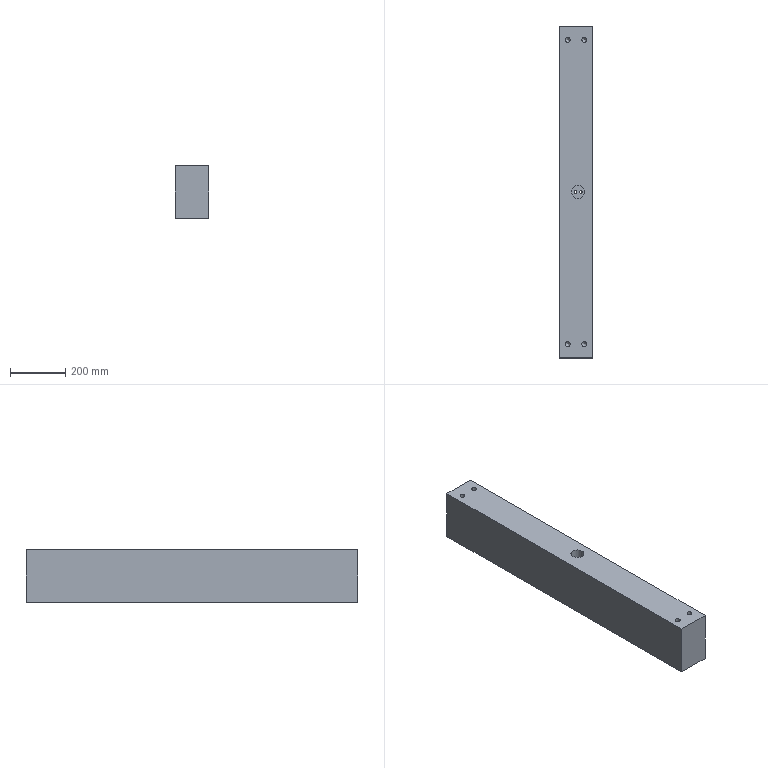Part | STEP file | lll_id4618_x_t | 1 solid | 30 faces | box 120 x 1200 x 190 mm | volume 27062039 mm3 | cylinder 13 | plane 9 | cone 8 | commonest cylinder face diameters 17.506 x8 9 x2 14 x2 47 x1
STEP:
#1=CARTESIAN_POINT('',(2746.188,550.,-370.));
#2=VERTEX_POINT('',#1);
#3=CARTESIAN_POINT('',(2737.435,550.,-370.));
#4=DIRECTION('',(0.,0.,1.));
#5=DIRECTION('',(1.,0.,0.));
#6=AXIS2_PLACEMENT_3D('',#3,#4,#5);
#7=CIRCLE('',#6,8.753);
#8=EDGE_CURVE('',#2,#2,#7,.T.);
#9=ORIENTED_EDGE('',*,*,#8,.T.);
#10=EDGE_LOOP('',(#9));
#11=FACE_BOUND('',#10,.T.);
#12=CARTESIAN_POINT('',(2746.188,-550.,-370.));
#13=VERTEX_POINT('',#12);
#14=CARTESIAN_POINT('',(2737.435,-550.,-370.));
#15=DIRECTION('',(0.,0.,1.));
#16=DIRECTION('',(1.,0.,0.));
#17=AXIS2_PLACEMENT_3D('',#14,#15,#16);
#18=CIRCLE('',#17,8.753);
#19=EDGE_CURVE('',#13,#13,#18,.T.);
#20=ORIENTED_EDGE('',*,*,#19,.T.);
#21=EDGE_LOOP('',(#20));
#22=FACE_BOUND('',#21,.T.);
#23=CARTESIAN_POINT('',(2698.,0.,-370.));
#24=VERTEX_POINT('',#23);
#25=CARTESIAN_POINT('',(2705.,0.,-370.));
#26=DIRECTION('',(0.,0.,1.));
#27=DIRECTION('',(-1.,0.,0.));
#28=AXIS2_PLACEMENT_3D('',#25,#26,#27);
#29=CIRCLE('',#28,7.);
#30=EDGE_CURVE('',#24,#24,#29,.T.);
#31=ORIENTED_EDGE('',*,*,#30,.T.);
#32=EDGE_LOOP('',(#31));
#33=FACE_BOUND('',#32,.T.);
#34=CARTESIAN_POINT('',(2647.435,600.,-370.));
#35=VERTEX_POINT('',#34);
#36=CARTESIAN_POINT('',(2647.435,-600.,-370.));
#37=VERTEX_POINT('',#36);
#38=CARTESIAN_POINT('',(2647.435,1.,-370.));
#39=DIRECTION('',(0.,-1.,0.));
#40=VECTOR('',#39,1.);
#41=LINE('',#38,#40);
#42=EDGE_CURVE('',#35,#37,#41,.T.);
#43=ORIENTED_EDGE('',*,*,#42,.F.);
#44=CARTESIAN_POINT('',(2767.435,600.,-370.));
#45=VERTEX_POINT('',#44);
#46=CARTESIAN_POINT('',(-1202.565,600.,-370.));
#47=DIRECTION('',(1.,0.,0.));
#48=VECTOR('',#47,1.);
#49=LINE('',#46,#48);
#50=EDGE_CURVE('',#35,#45,#49,.T.);
#51=ORIENTED_EDGE('',*,*,#50,.T.);
#52=CARTESIAN_POINT('',(2767.435,-600.,-370.));
#53=VERTEX_POINT('',#52);
#54=CARTESIAN_POINT('',(2767.435,600.,-370.));
#55=DIRECTION('',(0.,-1.,0.));
#56=VECTOR('',#55,1.);
#57=LINE('',#54,#56);
#58=EDGE_CURVE('',#45,#53,#57,.T.);
#59=ORIENTED_EDGE('',*,*,#58,.T.);
#60=CARTESIAN_POINT('',(2767.435,-600.,-370.));
#61=DIRECTION('',(-1.,0.,0.));
#62=VECTOR('',#61,1.);
#63=LINE('',#60,#62);
#64=EDGE_CURVE('',#53,#37,#63,.T.);
#65=ORIENTED_EDGE('',*,*,#64,.T.);
#66=EDGE_LOOP('',(#43,#51,#59,#65));
#67=FACE_BOUND('',#66,.T.);
#68=CARTESIAN_POINT('',(2718.,0.,-370.));
#69=VERTEX_POINT('',#68);
#70=CARTESIAN_POINT('',(2725.,0.,-370.));
#71=DIRECTION('',(0.,0.,1.));
#72=DIRECTION('',(-1.,0.,0.));
#73=AXIS2_PLACEMENT_3D('',#70,#71,#72);
#74=CIRCLE('',#73,7.);
#75=EDGE_CURVE('',#69,#69,#74,.T.);
#76=ORIENTED_EDGE('',*,*,#75,.T.);
#77=EDGE_LOOP('',(#76));
#78=FACE_BOUND('',#77,.T.);
#79=CARTESIAN_POINT('',(2686.188,550.,-370.));
#80=VERTEX_POINT('',#79);
#81=CARTESIAN_POINT('',(2677.435,550.,-370.));
#82=DIRECTION('',(0.,0.,1.));
#83=DIRECTION('',(1.,0.,0.));
#84=AXIS2_PLACEMENT_3D('',#81,#82,#83);
#85=CIRCLE('',#84,8.753);
#86=EDGE_CURVE('',#80,#80,#85,.T.);
#87=ORIENTED_EDGE('',*,*,#86,.T.);
#88=EDGE_LOOP('',(#87));
#89=FACE_BOUND('',#88,.T.);
#90=CARTESIAN_POINT('',(2686.188,-550.,-370.));
#91=VERTEX_POINT('',#90);
#92=CARTESIAN_POINT('',(2677.435,-550.,-370.));
#93=DIRECTION('',(0.,0.,1.));
#94=DIRECTION('',(1.,0.,0.));
#95=AXIS2_PLACEMENT_3D('',#92,#93,#94);
#96=CIRCLE('',#95,8.753);
#97=EDGE_CURVE('',#91,#91,#96,.T.);
#98=ORIENTED_EDGE('',*,*,#97,.T.);
#99=EDGE_LOOP('',(#98));
#100=FACE_BOUND('',#99,.T.);
#101=CARTESIAN_POINT('',(4953.751,1.,-370.));
#102=DIRECTION('',(0.,0.,-1.));
#103=DIRECTION('',(-1.,0.,0.));
#104=AXIS2_PLACEMENT_3D('',#101,#102,#103);
#105=PLANE('',#104);
#106=ADVANCED_FACE('',(#11,#22,#33,#67,#78,#89,#100),#105,.T.);
#107=CARTESIAN_POINT('',(2720.5,0.,-292.));
#108=VERTEX_POINT('',#107);
#109=CARTESIAN_POINT('',(2725.,0.,-292.));
#110=DIRECTION('',(0.,0.,-1.));
#111=DIRECTION('',(-1.,0.,0.));
#112=AXIS2_PLACEMENT_3D('',#109,#110,#111);
#113=CIRCLE('',#112,4.5);
#114=EDGE_CURVE('',#108,#108,#113,.T.);
#115=ORIENTED_EDGE('',*,*,#114,.F.);
#116=EDGE_LOOP('',(#115));
#117=FACE_BOUND('',#116,.T.);
#118=CARTESIAN_POINT('',(2720.5,0.,-322.));
#119=VERTEX_POINT('',#118);
#120=CARTESIAN_POINT('',(2725.,0.,-322.));
#121=DIRECTION('',(0.,0.,-1.));
#122=DIRECTION('',(-1.,0.,0.));
#123=AXIS2_PLACEMENT_3D('',#120,#121,#122);
#124=CIRCLE('',#123,4.5);
#125=EDGE_CURVE('',#119,#119,#124,.T.);
#126=ORIENTED_EDGE('',*,*,#125,.T.);
#127=EDGE_LOOP('',(#126));
#128=FACE_BOUND('',#127,.T.);
#129=CARTESIAN_POINT('',(2725.,0.,-432.));
#130=DIRECTION('',(0.,0.,1.));
#131=DIRECTION('',(1.,0.,0.));
#132=AXIS2_PLACEMENT_3D('',#129,#130,#131);
#133=CYLINDRICAL_SURFACE('',#132,4.5);
#134=ADVANCED_FACE('',(#117,#128),#133,.F.);
#135=CARTESIAN_POINT('',(2700.5,0.,-292.));
#136=VERTEX_POINT('',#135);
#137=CARTESIAN_POINT('',(2705.,0.,-292.));
#138=DIRECTION('',(0.,0.,1.));
#139=DIRECTION('',(-1.,0.,0.));
#140=AXIS2_PLACEMENT_3D('',#137,#138,#139);
#141=CIRCLE('',#140,4.5);
#142=EDGE_CURVE('',#136,#136,#141,.T.);
#143=ORIENTED_EDGE('',*,*,#142,.T.);
#144=EDGE_LOOP('',(#143));
#145=FACE_BOUND('',#144,.T.);
#146=CARTESIAN_POINT('',(2700.5,0.,-322.));
#147=VERTEX_POINT('',#146);
#148=CARTESIAN_POINT('',(2705.,0.,-322.));
#149=DIRECTION('',(0.,0.,1.));
#150=DIRECTION('',(-1.,0.,0.));
#151=AXIS2_PLACEMENT_3D('',#148,#149,#150);
#152=CIRCLE('',#151,4.5);
#153=EDGE_CURVE('',#147,#147,#152,.T.);
#154=ORIENTED_EDGE('',*,*,#153,.F.);
#155=EDGE_LOOP('',(#154));
#156=FACE_BOUND('',#155,.T.);
#157=CARTESIAN_POINT('',(2705.,0.,-432.));
#158=DIRECTION('',(0.,0.,1.));
#159=DIRECTION('',(1.,0.,0.));
#160=AXIS2_PLACEMENT_3D('',#157,#158,#159);
#161=CYLINDRICAL_SURFACE('',#160,4.5);
#162=ADVANCED_FACE('',(#145,#156),#161,.F.);
#163=CARTESIAN_POINT('',(2691.5,0.,-292.));
#164=VERTEX_POINT('',#163);
#165=CARTESIAN_POINT('',(2715.,0.,-292.));
#166=DIRECTION('',(0.,0.,-1.));
#167=DIRECTION('',(-1.,0.,0.));
#168=AXIS2_PLACEMENT_3D('',#165,#166,#167);
#169=CIRCLE('',#168,23.5);
#170=EDGE_CURVE('',#164,#164,#169,.T.);
#171=ORIENTED_EDGE('',*,*,#170,.F.);
#172=EDGE_LOOP('',(#171));
#173=FACE_BOUND('',#172,.T.);
#174=ORIENTED_EDGE('',*,*,#142,.F.);
#175=EDGE_LOOP('',(#174));
#176=FACE_BOUND('',#175,.T.);
#177=ORIENTED_EDGE('',*,*,#114,.T.);
#178=EDGE_LOOP('',(#177));
#179=FACE_BOUND('',#178,.T.);
#180=CARTESIAN_POINT('',(2725.8,0.,-292.));
#181=DIRECTION('',(0.,0.,-1.));
#182=DIRECTION('',(1.,0.,0.));
#183=AXIS2_PLACEMENT_3D('',#180,#181,#182);
#184=PLANE('',#183);
#185=ADVANCED_FACE('',(#173,#176,#179),#184,.F.);
#186=CARTESIAN_POINT('',(2668.682,550.,-180.));
#187=VERTEX_POINT('',#186);
#188=CARTESIAN_POINT('',(2677.435,550.,-180.));
#189=DIRECTION('',(0.,0.,-1.));
#190=DIRECTION('',(-1.,0.,0.));
#191=AXIS2_PLACEMENT_3D('',#188,#189,#190);
#192=CIRCLE('',#191,8.753);
#193=EDGE_CURVE('',#187,#187,#192,.T.);
#194=ORIENTED_EDGE('',*,*,#193,.T.);
#195=EDGE_LOOP('',(#194));
#196=FACE_BOUND('',#195,.T.);
#197=CARTESIAN_POINT('',(2668.682,-550.,-180.));
#198=VERTEX_POINT('',#197);
#199=CARTESIAN_POINT('',(2677.435,-550.,-180.));
#200=DIRECTION('',(0.,0.,-1.));
#201=DIRECTION('',(-1.,0.,0.));
#202=AXIS2_PLACEMENT_3D('',#199,#200,#201);
#203=CIRCLE('',#202,8.753);
#204=EDGE_CURVE('',#198,#198,#203,.T.);
#205=ORIENTED_EDGE('',*,*,#204,.T.);
#206=EDGE_LOOP('',(#205));
#207=FACE_BOUND('',#206,.T.);
#208=CARTESIAN_POINT('',(2728.682,-550.,-180.));
#209=VERTEX_POINT('',#208);
#210=CARTESIAN_POINT('',(2737.435,-550.,-180.));
#211=DIRECTION('',(0.,0.,-1.));
#212=DIRECTION('',(-1.,0.,0.));
#213=AXIS2_PLACEMENT_3D('',#210,#211,#212);
#214=CIRCLE('',#213,8.753);
#215=EDGE_CURVE('',#209,#209,#214,.T.);
#216=ORIENTED_EDGE('',*,*,#215,.T.);
#217=EDGE_LOOP('',(#216));
#218=FACE_BOUND('',#217,.T.);
#219=CARTESIAN_POINT('',(2728.682,550.,-180.));
#220=VERTEX_POINT('',#219);
#221=CARTESIAN_POINT('',(2737.435,550.,-180.));
#222=DIRECTION('',(0.,0.,-1.));
#223=DIRECTION('',(-1.,0.,0.));
#224=AXIS2_PLACEMENT_3D('',#221,#222,#223);
#225=CIRCLE('',#224,8.753);
#226=EDGE_CURVE('',#220,#220,#225,.T.);
#227=ORIENTED_EDGE('',*,*,#226,.T.);
#228=EDGE_LOOP('',(#227));
#229=FACE_BOUND('',#228,.T.);
#230=CARTESIAN_POINT('',(2647.435,600.,-180.));
#231=VERTEX_POINT('',#230);
#232=CARTESIAN_POINT('',(2767.435,600.,-180.));
#233=VERTEX_POINT('',#232);
#234=CARTESIAN_POINT('',(4953.751,600.,-180.));
#235=DIRECTION('',(1.,0.,0.));
#236=VECTOR('',#235,1.);
#237=LINE('',#234,#236);
#238=EDGE_CURVE('',#231,#233,#237,.T.);
#239=ORIENTED_EDGE('',*,*,#238,.F.);
#240=CARTESIAN_POINT('',(2647.435,-600.,-180.));
#241=VERTEX_POINT('',#240);
#242=CARTESIAN_POINT('',(2647.435,0.,-180.));
#243=DIRECTION('',(0.,1.,0.));
#244=VECTOR('',#243,1.);
#245=LINE('',#242,#244);
#246=EDGE_CURVE('',#241,#231,#245,.T.);
#247=ORIENTED_EDGE('',*,*,#246,.F.);
#248=CARTESIAN_POINT('',(2767.435,-600.,-180.));
#249=VERTEX_POINT('',#248);
#250=CARTESIAN_POINT('',(4953.751,-600.,-180.));
#251=DIRECTION('',(-1.,0.,0.));
#252=VECTOR('',#251,1.);
#253=LINE('',#250,#252);
#254=EDGE_CURVE('',#249,#241,#253,.T.);
#255=ORIENTED_EDGE('',*,*,#254,.F.);
#256=CARTESIAN_POINT('',(2767.435,1.,-180.));
#257=DIRECTION('',(0.,-1.,0.));
#258=VECTOR('',#257,1.);
#259=LINE('',#256,#258);
#260=EDGE_CURVE('',#233,#249,#259,.T.);
#261=ORIENTED_EDGE('',*,*,#260,.F.);
#262=EDGE_LOOP('',(#239,#247,#255,#261));
#263=FACE_BOUND('',#262,.T.);
#264=CARTESIAN_POINT('',(2691.5,0.,-180.));
#265=VERTEX_POINT('',#264);
#266=CARTESIAN_POINT('',(2715.,0.,-180.));
#267=DIRECTION('',(0.,0.,1.));
#268=DIRECTION('',(-1.,0.,0.));
#269=AXIS2_PLACEMENT_3D('',#266,#267,#268);
#270=CIRCLE('',#269,23.5);
#271=EDGE_CURVE('',#265,#265,#270,.T.);
#272=ORIENTED_EDGE('',*,*,#271,.F.);
#273=EDGE_LOOP('',(#272));
#274=FACE_BOUND('',#273,.T.);
#275=CARTESIAN_POINT('',(4953.751,1.,-180.));
#276=DIRECTION('',(0.,0.,-1.));
#277=DIRECTION('',(-1.,0.,0.));
#278=AXIS2_PLACEMENT_3D('',#275,#276,#277);
#279=PLANE('',#278);
#280=ADVANCED_FACE('',(#196,#207,#218,#229,#263,#274),#279,.F.);
#281=ORIENTED_EDGE('',*,*,#58,.F.);
#282=CARTESIAN_POINT('',(2767.435,600.,-182.5));
#283=DIRECTION('',(0.,0.,-1.));
#284=VECTOR('',#283,1.);
#285=LINE('',#282,#284);
#286=EDGE_CURVE('',#233,#45,#285,.T.);
#287=ORIENTED_EDGE('',*,*,#286,.F.);
#288=ORIENTED_EDGE('',*,*,#260,.T.);
#289=CARTESIAN_POINT('',(2767.435,-600.,-182.5));
#290=DIRECTION('',(0.,0.,-1.));
#291=VECTOR('',#290,1.);
#292=LINE('',#289,#291);
#293=EDGE_CURVE('',#249,#53,#292,.T.);
#294=ORIENTED_EDGE('',*,*,#293,.T.);
#295=EDGE_LOOP('',(#281,#287,#288,#294));
#296=FACE_OUTER_BOUND('',#295,.T.);
#297=CARTESIAN_POINT('',(2767.435,600.,-182.5));
#298=DIRECTION('',(1.,0.,0.));
#299=DIRECTION('',(0.,0.,-1.));
#300=AXIS2_PLACEMENT_3D('',#297,#298,#299);
#301=PLANE('',#300);
#302=ADVANCED_FACE('',(#296),#301,.T.);
#303=CARTESIAN_POINT('',(2647.435,-600.,-251.25));
#304=DIRECTION('',(0.,0.,-1.));
#305=VECTOR('',#304,1.);
#306=LINE('',#303,#305);
#307=EDGE_CURVE('',#241,#37,#306,.T.);
#308=ORIENTED_EDGE('',*,*,#307,.T.);
#309=ORIENTED_EDGE('',*,*,#64,.F.);
#310=ORIENTED_EDGE('',*,*,#293,.F.);
#311=ORIENTED_EDGE('',*,*,#254,.T.);
#312=EDGE_LOOP('',(#308,#309,#310,#311));
#313=FACE_OUTER_BOUND('',#312,.T.);
#314=CARTESIAN_POINT('',(2767.435,-600.,-182.5));
#315=DIRECTION('',(0.,-1.,0.));
#316=DIRECTION('',(0.,0.,-1.));
#317=AXIS2_PLACEMENT_3D('',#314,#315,#316);
#318=PLANE('',#317);
#319=ADVANCED_FACE('',(#313),#318,.T.);
#320=CARTESIAN_POINT('',(2647.435,600.,-251.25));
#321=DIRECTION('',(0.,0.,1.));
#322=VECTOR('',#321,1.);
#323=LINE('',#320,#322);
#324=EDGE_CURVE('',#35,#231,#323,.T.);
#325=ORIENTED_EDGE('',*,*,#324,.T.);
#326=ORIENTED_EDGE('',*,*,#238,.T.);
#327=ORIENTED_EDGE('',*,*,#286,.T.);
#328=ORIENTED_EDGE('',*,*,#50,.F.);
#329=EDGE_LOOP('',(#325,#326,#327,#328));
#330=FACE_OUTER_BOUND('',#329,.T.);
#331=CARTESIAN_POINT('',(-1202.565,600.,-182.5));
#332=DIRECTION('',(0.,1.,0.));
#333=DIRECTION('',(0.,0.,1.));
#334=AXIS2_PLACEMENT_3D('',#331,#332,#333);
#335=PLANE('',#334);
#336=ADVANCED_FACE('',(#330),#335,.T.);
#337=ORIENTED_EDGE('',*,*,#324,.F.);
#338=ORIENTED_EDGE('',*,*,#42,.T.);
#339=ORIENTED_EDGE('',*,*,#307,.F.);
#340=ORIENTED_EDGE('',*,*,#246,.T.);
#341=EDGE_LOOP('',(#337,#338,#339,#340));
#342=FACE_OUTER_BOUND('',#341,.T.);
#343=CARTESIAN_POINT('',(2647.435,0.,-251.25));
#344=DIRECTION('',(1.,0.,0.));
#345=DIRECTION('',(0.,0.,-1.));
#346=AXIS2_PLACEMENT_3D('',#343,#344,#345);
#347=PLANE('',#346);
#348=ADVANCED_FACE('',(#342),#347,.F.);
#349=ORIENTED_EDGE('',*,*,#170,.T.);
#350=EDGE_LOOP('',(#349));
#351=FACE_BOUND('',#350,.T.);
#352=ORIENTED_EDGE('',*,*,#271,.T.);
#353=EDGE_LOOP('',(#352));
#354=FACE_BOUND('',#353,.T.);
#355=CARTESIAN_POINT('',(2715.,0.,-288.));
#356=DIRECTION('',(0.,0.,1.));
#357=DIRECTION('',(1.,0.,0.));
#358=AXIS2_PLACEMENT_3D('',#355,#356,#357);
#359=CYLINDRICAL_SURFACE('',#358,23.5);
#360=ADVANCED_FACE('',(#351,#354),#359,.F.);
#361=CARTESIAN_POINT('',(2698.,0.,-322.));
#362=VERTEX_POINT('',#361);
#363=CARTESIAN_POINT('',(2705.,0.,-322.));
#364=DIRECTION('',(0.,0.,1.));
#365=DIRECTION('',(-1.,0.,0.));
#366=AXIS2_PLACEMENT_3D('',#363,#364,#365);
#367=CIRCLE('',#366,7.);
#368=EDGE_CURVE('',#362,#362,#367,.T.);
#369=ORIENTED_EDGE('',*,*,#368,.F.);
#370=EDGE_LOOP('',(#369));
#371=FACE_BOUND('',#370,.T.);
#372=ORIENTED_EDGE('',*,*,#153,.T.);
#373=EDGE_LOOP('',(#372));
#374=FACE_BOUND('',#373,.T.);
#375=CARTESIAN_POINT('',(2705.,0.,-322.));
#376=DIRECTION('',(0.,0.,-1.));
#377=DIRECTION('',(-1.,0.,0.));
#378=AXIS2_PLACEMENT_3D('',#375,#376,#377);
#379=PLANE('',#378);
#380=ADVANCED_FACE('',(#371,#374),#379,.T.);
#381=ORIENTED_EDGE('',*,*,#30,.F.);
#382=EDGE_LOOP('',(#381));
#383=FACE_BOUND('',#382,.T.);
#384=ORIENTED_EDGE('',*,*,#368,.T.);
#385=EDGE_LOOP('',(#384));
#386=FACE_BOUND('',#385,.T.);
#387=CARTESIAN_POINT('',(2705.,0.,-432.));
#388=DIRECTION('',(0.,0.,1.));
#389=DIRECTION('',(1.,0.,0.));
#390=AXIS2_PLACEMENT_3D('',#387,#388,#389);
#391=CYLINDRICAL_SURFACE('',#390,7.);
#392=ADVANCED_FACE('',(#383,#386),#391,.F.);
#393=ORIENTED_EDGE('',*,*,#75,.F.);
#394=EDGE_LOOP('',(#393));
#395=FACE_BOUND('',#394,.T.);
#396=CARTESIAN_POINT('',(2718.,0.,-322.));
#397=VERTEX_POINT('',#396);
#398=CARTESIAN_POINT('',(2725.,0.,-322.));
#399=DIRECTION('',(0.,0.,1.));
#400=DIRECTION('',(-1.,0.,0.));
#401=AXIS2_PLACEMENT_3D('',#398,#399,#400);
#402=CIRCLE('',#401,7.);
#403=EDGE_CURVE('',#397,#397,#402,.T.);
#404=ORIENTED_EDGE('',*,*,#403,.T.);
#405=EDGE_LOOP('',(#404));
#406=FACE_BOUND('',#405,.T.);
#407=CARTESIAN_POINT('',(2725.,0.,-432.));
#408=DIRECTION('',(0.,0.,1.));
#409=DIRECTION('',(1.,0.,0.));
#410=AXIS2_PLACEMENT_3D('',#407,#408,#409);
#411=CYLINDRICAL_SURFACE('',#410,7.);
#412=ADVANCED_FACE('',(#395,#406),#411,.F.);
#413=ORIENTED_EDGE('',*,*,#125,.F.);
#414=EDGE_LOOP('',(#413));
#415=FACE_BOUND('',#414,.T.);
#416=ORIENTED_EDGE('',*,*,#403,.F.);
#417=EDGE_LOOP('',(#416));
#418=FACE_BOUND('',#417,.T.);
#419=CARTESIAN_POINT('',(2725.,0.,-322.));
#420=DIRECTION('',(0.,0.,-1.));
#421=DIRECTION('',(-1.,0.,0.));
#422=AXIS2_PLACEMENT_3D('',#419,#420,#421);
#423=PLANE('',#422);
#424=ADVANCED_FACE('',(#415,#418),#423,.T.);
#425=CARTESIAN_POINT('',(2728.682,550.,-221.253));
#426=VERTEX_POINT('',#425);
#427=CARTESIAN_POINT('',(2737.435,550.,-221.253));
#428=DIRECTION('',(0.,0.,-1.));
#429=DIRECTION('',(-1.,0.,0.));
#430=AXIS2_PLACEMENT_3D('',#427,#428,#429);
#431=CIRCLE('',#430,8.753);
#432=EDGE_CURVE('',#426,#426,#431,.T.);
#433=ORIENTED_EDGE('',*,*,#432,.T.);
#434=EDGE_LOOP('',(#433));
#435=FACE_BOUND('',#434,.T.);
#436=ORIENTED_EDGE('',*,*,#226,.F.);
#437=EDGE_LOOP('',(#436));
#438=FACE_BOUND('',#437,.T.);
#439=CARTESIAN_POINT('',(2737.435,550.,-180.));
#440=DIRECTION('',(0.,0.,-1.));
#441=DIRECTION('',(1.,0.,0.));
#442=AXIS2_PLACEMENT_3D('',#439,#440,#441);
#443=CYLINDRICAL_SURFACE('',#442,8.753);
#444=ADVANCED_FACE('',(#435,#438),#443,.F.);
#445=CARTESIAN_POINT('',(2737.435,550.,-230.006));
#446=VERTEX_POINT('',#445);
#447=VERTEX_LOOP('',#446);
#448=FACE_BOUND('',#447,.T.);
#449=ORIENTED_EDGE('',*,*,#432,.F.);
#450=EDGE_LOOP('',(#449));
#451=FACE_BOUND('',#450,.T.);
#452=CARTESIAN_POINT('',(2737.435,550.,-221.253));
#453=DIRECTION('',(0.,0.,1.));
#454=DIRECTION('',(-1.,0.,0.));
#455=AXIS2_PLACEMENT_3D('',#452,#453,#454);
#456=CONICAL_SURFACE('',#455,8.753,45.);
#457=ADVANCED_FACE('',(#448,#451),#456,.F.);
#458=CARTESIAN_POINT('',(2728.682,-550.,-221.253));
#459=VERTEX_POINT('',#458);
#460=CARTESIAN_POINT('',(2737.435,-550.,-221.253));
#461=DIRECTION('',(0.,0.,-1.));
#462=DIRECTION('',(-1.,0.,0.));
#463=AXIS2_PLACEMENT_3D('',#460,#461,#462);
#464=CIRCLE('',#463,8.753);
#465=EDGE_CURVE('',#459,#459,#464,.T.);
#466=ORIENTED_EDGE('',*,*,#465,.T.);
#467=EDGE_LOOP('',(#466));
#468=FACE_BOUND('',#467,.T.);
#469=ORIENTED_EDGE('',*,*,#215,.F.);
#470=EDGE_LOOP('',(#469));
#471=FACE_BOUND('',#470,.T.);
#472=CARTESIAN_POINT('',(2737.435,-550.,-180.));
#473=DIRECTION('',(0.,0.,-1.));
#474=DIRECTION('',(1.,0.,0.));
#475=AXIS2_PLACEMENT_3D('',#472,#473,#474);
#476=CYLINDRICAL_SURFACE('',#475,8.753);
#477=ADVANCED_FACE('',(#468,#471),#476,.F.);
#478=CARTESIAN_POINT('',(2737.435,-550.,-230.006));
#479=VERTEX_POINT('',#478);
#480=VERTEX_LOOP('',#479);
#481=FACE_BOUND('',#480,.T.);
#482=ORIENTED_EDGE('',*,*,#465,.F.);
#483=EDGE_LOOP('',(#482));
#484=FACE_BOUND('',#483,.T.);
#485=CARTESIAN_POINT('',(2737.435,-550.,-221.253));
#486=DIRECTION('',(0.,0.,1.));
#487=DIRECTION('',(-1.,0.,0.));
#488=AXIS2_PLACEMENT_3D('',#485,#486,#487);
#489=CONICAL_SURFACE('',#488,8.753,45.);
#490=ADVANCED_FACE('',(#481,#484),#489,.F.);
#491=CARTESIAN_POINT('',(2668.682,-550.,-221.253));
#492=VERTEX_POINT('',#491);
#493=CARTESIAN_POINT('',(2677.435,-550.,-221.253));
#494=DIRECTION('',(0.,0.,-1.));
#495=DIRECTION('',(-1.,0.,0.));
#496=AXIS2_PLACEMENT_3D('',#493,#494,#495);
#497=CIRCLE('',#496,8.753);
#498=EDGE_CURVE('',#492,#492,#497,.T.);
#499=ORIENTED_EDGE('',*,*,#498,.T.);
#500=EDGE_LOOP('',(#499));
#501=FACE_BOUND('',#500,.T.);
#502=ORIENTED_EDGE('',*,*,#204,.F.);
#503=EDGE_LOOP('',(#502));
#504=FACE_BOUND('',#503,.T.);
#505=CARTESIAN_POINT('',(2677.435,-550.,-180.));
#506=DIRECTION('',(0.,0.,-1.));
#507=DIRECTION('',(1.,0.,0.));
#508=AXIS2_PLACEMENT_3D('',#505,#506,#507);
#509=CYLINDRICAL_SURFACE('',#508,8.753);
#510=ADVANCED_FACE('',(#501,#504),#509,.F.);
#511=CARTESIAN_POINT('',(2677.435,-550.,-230.006));
#512=VERTEX_POINT('',#511);
#513=VERTEX_LOOP('',#512);
#514=FACE_BOUND('',#513,.T.);
#515=ORIENTED_EDGE('',*,*,#498,.F.);
#516=EDGE_LOOP('',(#515));
#517=FACE_BOUND('',#516,.T.);
#518=CARTESIAN_POINT('',(2677.435,-550.,-221.253));
#519=DIRECTION('',(0.,0.,1.));
#520=DIRECTION('',(-1.,0.,0.));
#521=AXIS2_PLACEMENT_3D('',#518,#519,#520);
#522=CONICAL_SURFACE('',#521,8.753,45.);
#523=ADVANCED_FACE('',(#514,#517),#522,.F.);
#524=CARTESIAN_POINT('',(2668.682,550.,-221.253));
#525=VERTEX_POINT('',#524);
#526=CARTESIAN_POINT('',(2677.435,550.,-221.253));
#527=DIRECTION('',(0.,0.,-1.));
#528=DIRECTION('',(-1.,0.,0.));
#529=AXIS2_PLACEMENT_3D('',#526,#527,#528);
#530=CIRCLE('',#529,8.753);
#531=EDGE_CURVE('',#525,#525,#530,.T.);
#532=ORIENTED_EDGE('',*,*,#531,.T.);
#533=EDGE_LOOP('',(#532));
#534=FACE_BOUND('',#533,.T.);
#535=ORIENTED_EDGE('',*,*,#193,.F.);
#536=EDGE_LOOP('',(#535));
#537=FACE_BOUND('',#536,.T.);
#538=CARTESIAN_POINT('',(2677.435,550.,-180.));
#539=DIRECTION('',(0.,0.,-1.));
#540=DIRECTION('',(1.,0.,0.));
#541=AXIS2_PLACEMENT_3D('',#538,#539,#540);
#542=CYLINDRICAL_SURFACE('',#541,8.753);
#543=ADVANCED_FACE('',(#534,#537),#542,.F.);
#544=CARTESIAN_POINT('',(2677.435,550.,-230.006));
#545=VERTEX_POINT('',#544);
#546=VERTEX_LOOP('',#545);
#547=FACE_BOUND('',#546,.T.);
#548=ORIENTED_EDGE('',*,*,#531,.F.);
#549=EDGE_LOOP('',(#548));
#550=FACE_BOUND('',#549,.T.);
#551=CARTESIAN_POINT('',(2677.435,550.,-221.253));
#552=DIRECTION('',(0.,0.,1.));
#553=DIRECTION('',(-1.,0.,0.));
#554=AXIS2_PLACEMENT_3D('',#551,#552,#553);
#555=CONICAL_SURFACE('',#554,8.753,45.);
#556=ADVANCED_FACE('',(#547,#550),#555,.F.);
#557=CARTESIAN_POINT('',(2746.188,-550.,-328.747));
#558=VERTEX_POINT('',#557);
#559=CARTESIAN_POINT('',(2737.435,-550.,-328.747));
#560=DIRECTION('',(0.,0.,1.));
#561=DIRECTION('',(1.,0.,0.));
#562=AXIS2_PLACEMENT_3D('',#559,#560,#561);
#563=CIRCLE('',#562,8.753);
#564=EDGE_CURVE('',#558,#558,#563,.T.);
#565=ORIENTED_EDGE('',*,*,#564,.T.);
#566=EDGE_LOOP('',(#565));
#567=FACE_BOUND('',#566,.T.);
#568=ORIENTED_EDGE('',*,*,#19,.F.);
#569=EDGE_LOOP('',(#568));
#570=FACE_BOUND('',#569,.T.);
#571=CARTESIAN_POINT('',(2737.435,-550.,-370.));
#572=DIRECTION('',(0.,0.,1.));
#573=DIRECTION('',(-1.,0.,0.));
#574=AXIS2_PLACEMENT_3D('',#571,#572,#573);
#575=CYLINDRICAL_SURFACE('',#574,8.753);
#576=ADVANCED_FACE('',(#567,#570),#575,.F.);
#577=CARTESIAN_POINT('',(2737.435,-550.,-319.994));
#578=VERTEX_POINT('',#577);
#579=VERTEX_LOOP('',#578);
#580=FACE_BOUND('',#579,.T.);
#581=ORIENTED_EDGE('',*,*,#564,.F.);
#582=EDGE_LOOP('',(#581));
#583=FACE_BOUND('',#582,.T.);
#584=CARTESIAN_POINT('',(2737.435,-550.,-328.747));
#585=DIRECTION('',(0.,0.,-1.));
#586=DIRECTION('',(1.,0.,0.));
#587=AXIS2_PLACEMENT_3D('',#584,#585,#586);
#588=CONICAL_SURFACE('',#587,8.753,45.);
#589=ADVANCED_FACE('',(#580,#583),#588,.F.);
#590=CARTESIAN_POINT('',(2686.188,550.,-328.747));
#591=VERTEX_POINT('',#590);
#592=CARTESIAN_POINT('',(2677.435,550.,-328.747));
#593=DIRECTION('',(0.,0.,1.));
#594=DIRECTION('',(1.,0.,0.));
#595=AXIS2_PLACEMENT_3D('',#592,#593,#594);
#596=CIRCLE('',#595,8.753);
#597=EDGE_CURVE('',#591,#591,#596,.T.);
#598=ORIENTED_EDGE('',*,*,#597,.T.);
#599=EDGE_LOOP('',(#598));
#600=FACE_BOUND('',#599,.T.);
#601=ORIENTED_EDGE('',*,*,#86,.F.);
#602=EDGE_LOOP('',(#601));
#603=FACE_BOUND('',#602,.T.);
#604=CARTESIAN_POINT('',(2677.435,550.,-370.));
#605=DIRECTION('',(0.,0.,1.));
#606=DIRECTION('',(-1.,0.,0.));
#607=AXIS2_PLACEMENT_3D('',#604,#605,#606);
#608=CYLINDRICAL_SURFACE('',#607,8.753);
#609=ADVANCED_FACE('',(#600,#603),#608,.F.);
#610=CARTESIAN_POINT('',(2677.435,550.,-319.994));
#611=VERTEX_POINT('',#610);
#612=VERTEX_LOOP('',#611);
#613=FACE_BOUND('',#612,.T.);
#614=ORIENTED_EDGE('',*,*,#597,.F.);
#615=EDGE_LOOP('',(#614));
#616=FACE_BOUND('',#615,.T.);
#617=CARTESIAN_POINT('',(2677.435,550.,-328.747));
#618=DIRECTION('',(0.,0.,-1.));
#619=DIRECTION('',(1.,0.,0.));
#620=AXIS2_PLACEMENT_3D('',#617,#618,#619);
#621=CONICAL_SURFACE('',#620,8.753,45.);
#622=ADVANCED_FACE('',(#613,#616),#621,.F.);
#623=CARTESIAN_POINT('',(2746.188,550.,-328.747));
#624=VERTEX_POINT('',#623);
#625=CARTESIAN_POINT('',(2737.435,550.,-328.747));
#626=DIRECTION('',(0.,0.,1.));
#627=DIRECTION('',(1.,0.,0.));
#628=AXIS2_PLACEMENT_3D('',#625,#626,#627);
#629=CIRCLE('',#628,8.753);
#630=EDGE_CURVE('',#624,#624,#629,.T.);
#631=ORIENTED_EDGE('',*,*,#630,.T.);
#632=EDGE_LOOP('',(#631));
#633=FACE_BOUND('',#632,.T.);
#634=ORIENTED_EDGE('',*,*,#8,.F.);
#635=EDGE_LOOP('',(#634));
#636=FACE_BOUND('',#635,.T.);
#637=CARTESIAN_POINT('',(2737.435,550.,-370.));
#638=DIRECTION('',(0.,0.,1.));
#639=DIRECTION('',(-1.,0.,0.));
#640=AXIS2_PLACEMENT_3D('',#637,#638,#639);
#641=CYLINDRICAL_SURFACE('',#640,8.753);
#642=ADVANCED_FACE('',(#633,#636),#641,.F.);
#643=CARTESIAN_POINT('',(2737.435,550.,-319.994));
#644=VERTEX_POINT('',#643);
#645=VERTEX_LOOP('',#644);
#646=FACE_BOUND('',#645,.T.);
#647=ORIENTED_EDGE('',*,*,#630,.F.);
#648=EDGE_LOOP('',(#647));
#649=FACE_BOUND('',#648,.T.);
#650=CARTESIAN_POINT('',(2737.435,550.,-328.747));
#651=DIRECTION('',(0.,0.,-1.));
#652=DIRECTION('',(1.,0.,0.));
#653=AXIS2_PLACEMENT_3D('',#650,#651,#652);
#654=CONICAL_SURFACE('',#653,8.753,45.);
#655=ADVANCED_FACE('',(#646,#649),#654,.F.);
#656=CARTESIAN_POINT('',(2686.188,-550.,-328.747));
#657=VERTEX_POINT('',#656);
#658=CARTESIAN_POINT('',(2677.435,-550.,-328.747));
#659=DIRECTION('',(0.,0.,1.));
#660=DIRECTION('',(1.,0.,0.));
#661=AXIS2_PLACEMENT_3D('',#658,#659,#660);
#662=CIRCLE('',#661,8.753);
#663=EDGE_CURVE('',#657,#657,#662,.T.);
#664=ORIENTED_EDGE('',*,*,#663,.T.);
#665=EDGE_LOOP('',(#664));
#666=FACE_BOUND('',#665,.T.);
#667=ORIENTED_EDGE('',*,*,#97,.F.);
#668=EDGE_LOOP('',(#667));
#669=FACE_BOUND('',#668,.T.);
#670=CARTESIAN_POINT('',(2677.435,-550.,-370.));
#671=DIRECTION('',(0.,0.,1.));
#672=DIRECTION('',(-1.,0.,0.));
#673=AXIS2_PLACEMENT_3D('',#670,#671,#672);
#674=CYLINDRICAL_SURFACE('',#673,8.753);
#675=ADVANCED_FACE('',(#666,#669),#674,.F.);
#676=CARTESIAN_POINT('',(2677.435,-550.,-319.994));
#677=VERTEX_POINT('',#676);
#678=VERTEX_LOOP('',#677);
#679=FACE_BOUND('',#678,.T.);
#680=ORIENTED_EDGE('',*,*,#663,.F.);
#681=EDGE_LOOP('',(#680));
#682=FACE_BOUND('',#681,.T.);
#683=CARTESIAN_POINT('',(2677.435,-550.,-328.747));
#684=DIRECTION('',(0.,0.,-1.));
#685=DIRECTION('',(1.,0.,0.));
#686=AXIS2_PLACEMENT_3D('',#683,#684,#685);
#687=CONICAL_SURFACE('',#686,8.753,45.);
#688=ADVANCED_FACE('',(#679,#682),#687,.F.);
#689=CLOSED_SHELL('',(#106,#134,#162,#185,#280,#302,#319,#336,#348,#360,#380,#392,#412,#424,#444,#457,#477,#490,#510,#523,#543,#556,#576,#589,#609,#622,#642,#655,#675,#688));
#690=MANIFOLD_SOLID_BREP('',#689);
#691=(LENGTH_UNIT()NAMED_UNIT(*)SI_UNIT(.MILLI.,.METRE.));
#692=UNCERTAINTY_MEASURE_WITH_UNIT(LENGTH_MEASURE(0.00002),#691,'','');
#693=(NAMED_UNIT(*)PLANE_ANGLE_UNIT()SI_UNIT($,.RADIAN.));
#694=PLANE_ANGLE_MEASURE_WITH_UNIT(PLANE_ANGLE_MEASURE(0.01745),#693);
#695=DIMENSIONAL_EXPONENTS(0.,0.,0.,0.,0.,0.,0.);
#696=(CONVERSION_BASED_UNIT('DEGREE',#694)NAMED_UNIT(#695)PLANE_ANGLE_UNIT());
#697=(NAMED_UNIT(*)SI_UNIT($,.STERADIAN.)SOLID_ANGLE_UNIT());
#698=(GEOMETRIC_REPRESENTATION_CONTEXT(3)GLOBAL_UNCERTAINTY_ASSIGNED_CONTEXT((#692))GLOBAL_UNIT_ASSIGNED_CONTEXT((#691,#696,#697))REPRESENTATION_CONTEXT('',''));
#699=ADVANCED_BREP_SHAPE_REPRESENTATION('',(#690),#698);